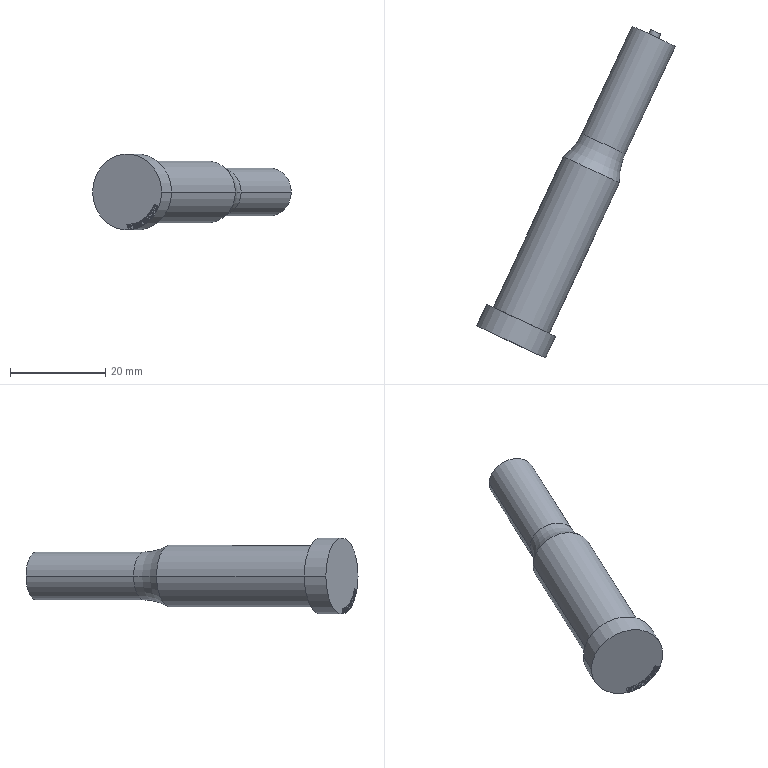Part | STEP file | 1_id22_x_t | 1 solid | 194 faces | box 41.811 x 69.852 x 16 mm | volume 8212 mm3 | plane 141 | other 43 | cylinder 8 | torus 2 | commonest cylinder face diameters 2.26 x2 10.05 x2 13 x2 16 x2